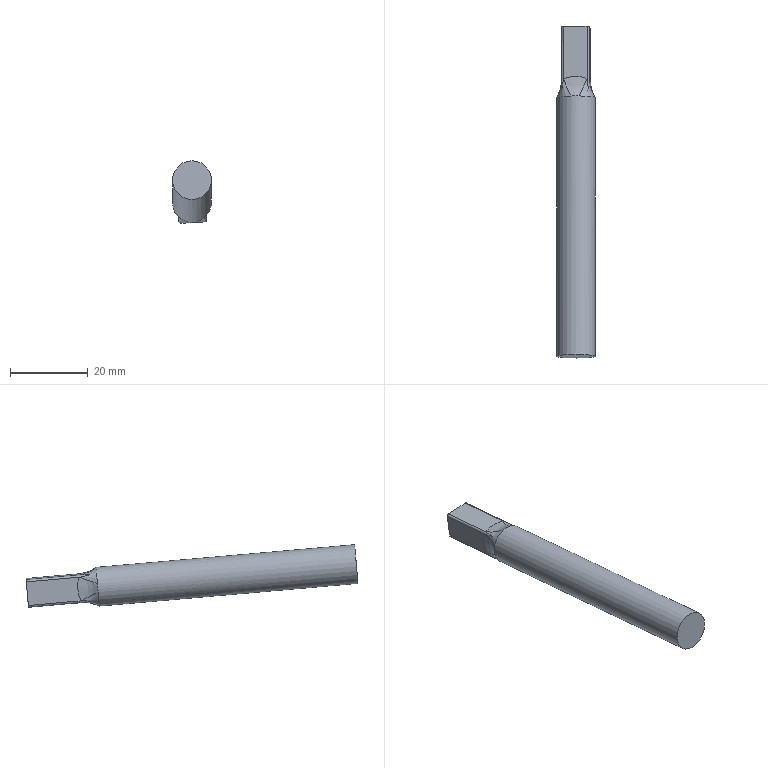Part | NX | features SPRS 10-80-7.100-7.100 2 | 1 solid | 19 faces | box 10 x 85.436 x 16.095 mm | volume 6207 mm3 | spline 8 | plane 6 | cylinder 5 | commonest cylinder face diameters 1 x4 10 x1
STEP:
#1=CARTESIAN_POINT('',(-225.118,-53.512,-35.743));
#2=VERTEX_POINT('',#1);
#3=CARTESIAN_POINT('',(-225.118,-67.066,-34.557));
#4=VERTEX_POINT('',#3);
#5=CARTESIAN_POINT('',(-225.118,-71.629,-34.158));
#6=DIRECTION('',(0.,0.9962,-0.08716));
#7=VECTOR('',#6,1000.);
#8=LINE('',#5,#7);
#9=EDGE_CURVE('',#2,#4,#8,.F.);
#10=ORIENTED_EDGE('',*,*,#9,.T.);
#11=CARTESIAN_POINT('',(-231.208,-67.096,-34.904));
#12=VERTEX_POINT('',#11);
#13=CARTESIAN_POINT('',(-225.118,-67.066,-34.557));
#14=CARTESIAN_POINT('',(-227.051,-66.254,-34.739));
#15=CARTESIAN_POINT('',(-229.277,-66.265,-34.866));
#16=CARTESIAN_POINT('',(-231.208,-67.096,-34.904));
#17=B_SPLINE_CURVE_WITH_KNOTS('',3,(#13,#14,#15,#16),.UNSPECIFIED.,.F.,.F.,(4,4),(0.,0.006313),.UNSPECIFIED.);
#18=EDGE_CURVE('',#4,#12,#17,.T.);
#19=ORIENTED_EDGE('',*,*,#18,.T.);
#20=CARTESIAN_POINT('',(-231.208,-53.543,-36.09));
#21=VERTEX_POINT('',#20);
#22=CARTESIAN_POINT('',(-231.208,-71.66,-34.505));
#23=DIRECTION('',(0.,0.9962,-0.08716));
#24=VECTOR('',#23,1000.);
#25=LINE('',#22,#24);
#26=EDGE_CURVE('',#12,#21,#25,.T.);
#27=ORIENTED_EDGE('',*,*,#26,.T.);
#28=CARTESIAN_POINT('',(-231.708,-53.545,-36.119));
#29=DIRECTION('',(0.9984,0.004985,0.05697));
#30=VECTOR('',#29,1000.);
#31=LINE('',#28,#30);
#32=EDGE_CURVE('',#21,#2,#31,.T.);
#33=ORIENTED_EDGE('',*,*,#32,.T.);
#34=EDGE_LOOP('',(#10,#19,#27,#33));
#35=FACE_BOUND('',#34,.T.);
#36=CARTESIAN_POINT('',(-231.708,-71.662,-34.534));
#37=DIRECTION('',(-0.05719,0.08701,0.9946));
#38=DIRECTION('',(0.,-0.9962,0.08716));
#39=AXIS2_PLACEMENT_3D('',#36,#37,#38);
#40=PLANE('',#39);
#41=ADVANCED_FACE('',(#35),#40,.F.);
#42=CARTESIAN_POINT('',(-224.997,-52.935,-29.15));
#43=VERTEX_POINT('',#42);
#44=CARTESIAN_POINT('',(-224.997,-66.489,-27.964));
#45=VERTEX_POINT('',#44);
#46=CARTESIAN_POINT('',(-224.997,-71.053,-27.565));
#47=DIRECTION('',(0.,0.9962,-0.08716));
#48=VECTOR('',#47,1000.);
#49=LINE('',#46,#48);
#50=EDGE_CURVE('',#43,#45,#49,.F.);
#51=ORIENTED_EDGE('',*,*,#50,.T.);
#52=CARTESIAN_POINT('',(-224.648,-67.02,-34.031));
#53=VERTEX_POINT('',#52);
#54=CARTESIAN_POINT('',(-224.997,-66.489,-27.964));
#55=CARTESIAN_POINT('',(-224.886,-65.836,-29.962));
#56=CARTESIAN_POINT('',(-224.758,-66.03,-32.179));
#57=CARTESIAN_POINT('',(-224.648,-67.02,-34.031));
#58=B_SPLINE_CURVE_WITH_KNOTS('',3,(#54,#55,#56,#57),.UNSPECIFIED.,.F.,.F.,(4,4),(0.,0.006313),.UNSPECIFIED.);
#59=EDGE_CURVE('',#45,#53,#58,.T.);
#60=ORIENTED_EDGE('',*,*,#59,.T.);
#61=CARTESIAN_POINT('',(-224.648,-53.466,-35.217));
#62=VERTEX_POINT('',#61);
#63=CARTESIAN_POINT('',(-224.648,-53.466,-35.217));
#64=DIRECTION('',(0.,0.9962,-0.08716));
#65=VECTOR('',#64,1000.);
#66=LINE('',#63,#65);
#67=EDGE_CURVE('',#53,#62,#66,.T.);
#68=ORIENTED_EDGE('',*,*,#67,.T.);
#69=CARTESIAN_POINT('',(-225.025,-52.892,-28.653));
#70=DIRECTION('',(0.05719,-0.08701,-0.9946));
#71=VECTOR('',#70,1000.);
#72=LINE('',#69,#71);
#73=EDGE_CURVE('',#43,#62,#72,.T.);
#74=ORIENTED_EDGE('',*,*,#73,.F.);
#75=EDGE_LOOP('',(#51,#60,#68,#74));
#76=FACE_BOUND('',#75,.T.);
#77=CARTESIAN_POINT('',(-225.025,-71.009,-27.068));
#78=DIRECTION('',(0.9984,0.004985,0.05697));
#79=DIRECTION('',(0.05698,0.,-0.9984));
#80=AXIS2_PLACEMENT_3D('',#77,#78,#79);
#81=PLANE('',#80);
#82=ADVANCED_FACE('',(#76),#81,.T.);
#83=CARTESIAN_POINT('',(-231.614,-52.925,-29.029));
#84=VERTEX_POINT('',#83);
#85=CARTESIAN_POINT('',(-231.614,-66.478,-27.843));
#86=VERTEX_POINT('',#85);
#87=CARTESIAN_POINT('',(-231.614,-71.042,-27.444));
#88=DIRECTION('',(0.,0.9962,-0.08716));
#89=VECTOR('',#88,1000.);
#90=LINE('',#87,#89);
#91=EDGE_CURVE('',#84,#86,#90,.F.);
#92=ORIENTED_EDGE('',*,*,#91,.T.);
#93=CARTESIAN_POINT('',(-225.524,-66.448,-27.495));
#94=VERTEX_POINT('',#93);
#95=CARTESIAN_POINT('',(-231.614,-66.478,-27.843));
#96=CARTESIAN_POINT('',(-229.682,-65.647,-27.805));
#97=CARTESIAN_POINT('',(-227.456,-65.636,-27.678));
#98=CARTESIAN_POINT('',(-225.524,-66.448,-27.495));
#99=B_SPLINE_CURVE_WITH_KNOTS('',3,(#95,#96,#97,#98),.UNSPECIFIED.,.F.,.F.,(4,4),(0.,0.006313),.UNSPECIFIED.);
#100=EDGE_CURVE('',#86,#94,#99,.T.);
#101=ORIENTED_EDGE('',*,*,#100,.T.);
#102=CARTESIAN_POINT('',(-225.524,-52.894,-28.681));
#103=VERTEX_POINT('',#102);
#104=CARTESIAN_POINT('',(-225.524,-52.894,-28.681));
#105=DIRECTION('',(0.,0.9962,-0.08716));
#106=VECTOR('',#105,1000.);
#107=LINE('',#104,#106);
#108=EDGE_CURVE('',#94,#103,#107,.T.);
#109=ORIENTED_EDGE('',*,*,#108,.T.);
#110=CARTESIAN_POINT('',(-225.025,-52.892,-28.653));
#111=DIRECTION('',(-0.9984,-0.004985,-0.05697));
#112=VECTOR('',#111,1000.);
#113=LINE('',#110,#112);
#114=EDGE_CURVE('',#103,#84,#113,.T.);
#115=ORIENTED_EDGE('',*,*,#114,.T.);
#116=EDGE_LOOP('',(#92,#101,#109,#115));
#117=FACE_BOUND('',#116,.T.);
#118=CARTESIAN_POINT('',(-225.025,-71.009,-27.068));
#119=DIRECTION('',(0.05719,-0.08701,-0.9946));
#120=DIRECTION('',(0.,0.9962,-0.08716));
#121=AXIS2_PLACEMENT_3D('',#118,#119,#120);
#122=PLANE('',#121);
#123=ADVANCED_FACE('',(#117),#122,.F.);
#124=CARTESIAN_POINT('',(-231.736,-53.502,-35.621));
#125=VERTEX_POINT('',#124);
#126=CARTESIAN_POINT('',(-231.736,-67.055,-34.436));
#127=VERTEX_POINT('',#126);
#128=CARTESIAN_POINT('',(-231.736,-71.619,-34.036));
#129=DIRECTION('',(0.,0.9962,-0.08716));
#130=VECTOR('',#129,1000.);
#131=LINE('',#128,#130);
#132=EDGE_CURVE('',#125,#127,#131,.F.);
#133=ORIENTED_EDGE('',*,*,#132,.T.);
#134=CARTESIAN_POINT('',(-232.085,-66.524,-28.369));
#135=VERTEX_POINT('',#134);
#136=CARTESIAN_POINT('',(-231.736,-67.055,-34.436));
#137=CARTESIAN_POINT('',(-231.847,-66.065,-32.582));
#138=CARTESIAN_POINT('',(-231.974,-65.872,-30.365));
#139=CARTESIAN_POINT('',(-232.085,-66.524,-28.369));
#140=B_SPLINE_CURVE_WITH_KNOTS('',3,(#136,#137,#138,#139),.UNSPECIFIED.,.F.,.F.,(4,4),(0.,0.006313),.UNSPECIFIED.);
#141=EDGE_CURVE('',#127,#135,#140,.T.);
#142=ORIENTED_EDGE('',*,*,#141,.T.);
#143=CARTESIAN_POINT('',(-232.085,-52.971,-29.555));
#144=VERTEX_POINT('',#143);
#145=CARTESIAN_POINT('',(-232.085,-71.088,-27.97));
#146=DIRECTION('',(0.,0.9962,-0.08716));
#147=VECTOR('',#146,1000.);
#148=LINE('',#145,#147);
#149=EDGE_CURVE('',#135,#144,#148,.T.);
#150=ORIENTED_EDGE('',*,*,#149,.T.);
#151=CARTESIAN_POINT('',(-232.114,-52.927,-29.057));
#152=DIRECTION('',(0.05719,-0.08701,-0.9946));
#153=VECTOR('',#152,1000.);
#154=LINE('',#151,#153);
#155=EDGE_CURVE('',#144,#125,#154,.T.);
#156=ORIENTED_EDGE('',*,*,#155,.T.);
#157=EDGE_LOOP('',(#133,#142,#150,#156));
#158=FACE_BOUND('',#157,.T.);
#159=CARTESIAN_POINT('',(-232.114,-71.044,-27.472));
#160=DIRECTION('',(0.9984,0.004985,0.05697));
#161=DIRECTION('',(0.05698,0.,-0.9984));
#162=AXIS2_PLACEMENT_3D('',#159,#160,#161);
#163=PLANE('',#162);
#164=ADVANCED_FACE('',(#158),#163,.F.);
#165=ORIENTED_EDGE('',*,*,#73,.T.);
#166=CARTESIAN_POINT('',(-225.147,-53.469,-35.245));
#167=DIRECTION('',(0.,0.9962,-0.08716));
#168=DIRECTION('',(0.,0.08716,0.9962));
#169=AXIS2_PLACEMENT_3D('',#166,#167,#168);
#170=CIRCLE('',#169,0.5);
#171=EDGE_CURVE('',#62,#2,#170,.T.);
#172=ORIENTED_EDGE('',*,*,#171,.T.);
#173=ORIENTED_EDGE('',*,*,#32,.F.);
#174=CARTESIAN_POINT('',(-231.237,-53.499,-35.593));
#175=DIRECTION('',(0.,0.9962,-0.08716));
#176=DIRECTION('',(0.,0.08716,0.9962));
#177=AXIS2_PLACEMENT_3D('',#174,#175,#176);
#178=CIRCLE('',#177,0.5);
#179=EDGE_CURVE('',#21,#125,#178,.T.);
#180=ORIENTED_EDGE('',*,*,#179,.T.);
#181=ORIENTED_EDGE('',*,*,#155,.F.);
#182=CARTESIAN_POINT('',(-231.586,-52.968,-29.526));
#183=DIRECTION('',(0.,0.9962,-0.08716));
#184=DIRECTION('',(0.,0.08716,0.9962));
#185=AXIS2_PLACEMENT_3D('',#182,#183,#184);
#186=CIRCLE('',#185,0.5);
#187=EDGE_CURVE('',#144,#84,#186,.T.);
#188=ORIENTED_EDGE('',*,*,#187,.T.);
#189=ORIENTED_EDGE('',*,*,#114,.F.);
#190=CARTESIAN_POINT('',(-225.496,-52.938,-29.179));
#191=DIRECTION('',(0.,0.9962,-0.08716));
#192=DIRECTION('',(0.,0.08716,0.9962));
#193=AXIS2_PLACEMENT_3D('',#190,#191,#192);
#194=CIRCLE('',#193,0.5);
#195=EDGE_CURVE('',#103,#43,#194,.T.);
#196=ORIENTED_EDGE('',*,*,#195,.T.);
#197=EDGE_LOOP('',(#165,#172,#173,#180,#181,#188,#189,#196));
#198=FACE_BOUND('',#197,.T.);
#199=CARTESIAN_POINT('',(-231.708,-53.545,-36.119));
#200=DIRECTION('',(0.,0.9962,-0.08716));
#201=DIRECTION('',(0.,0.08716,0.9962));
#202=AXIS2_PLACEMENT_3D('',#199,#200,#201);
#203=PLANE('',#202);
#204=ADVANCED_FACE('',(#198),#203,.T.);
#205=CARTESIAN_POINT('',(-228.366,-138.331,-29.958));
#206=VERTEX_POINT('',#205);
#207=CARTESIAN_POINT('',(-228.366,-137.895,-24.977));
#208=DIRECTION('',(0.,-0.9962,0.08716));
#209=DIRECTION('',(0.,-0.08716,-0.9962));
#210=AXIS2_PLACEMENT_3D('',#207,#208,#209);
#211=CIRCLE('',#210,5.);
#212=EDGE_CURVE('',#206,#206,#211,.F.);
#213=ORIENTED_EDGE('',*,*,#212,.F.);
#214=EDGE_LOOP('',(#213));
#215=FACE_BOUND('',#214,.T.);
#216=CARTESIAN_POINT('',(-228.366,-137.895,-24.977));
#217=DIRECTION('',(0.,-0.9962,0.08716));
#218=DIRECTION('',(0.,-0.08716,-0.9962));
#219=AXIS2_PLACEMENT_3D('',#216,#217,#218);
#220=PLANE('',#219);
#221=ADVANCED_FACE('',(#215),#220,.T.);
#222=ORIENTED_EDGE('',*,*,#212,.T.);
#223=EDGE_LOOP('',(#222));
#224=FACE_BOUND('',#223,.T.);
#225=CARTESIAN_POINT('',(-226.991,-71.755,-35.59));
#226=VERTEX_POINT('',#225);
#227=CARTESIAN_POINT('',(-223.434,-71.407,-31.615));
#228=VERTEX_POINT('',#227);
#229=CARTESIAN_POINT('',(-228.366,-71.336,-30.801));
#230=DIRECTION('',(0.,-0.9962,0.08716));
#231=DIRECTION('',(0.,-0.08716,-0.9962));
#232=AXIS2_PLACEMENT_3D('',#229,#230,#231);
#233=CIRCLE('',#232,5.);
#234=EDGE_CURVE('',#226,#228,#233,.T.);
#235=ORIENTED_EDGE('',*,*,#234,.T.);
#236=CARTESIAN_POINT('',(-223.559,-71.216,-29.431));
#237=VERTEX_POINT('',#236);
#238=CARTESIAN_POINT('',(-228.366,-71.336,-30.801));
#239=DIRECTION('',(0.,-0.9962,0.08716));
#240=DIRECTION('',(0.,-0.08716,-0.9962));
#241=AXIS2_PLACEMENT_3D('',#238,#239,#240);
#242=CIRCLE('',#241,5.);
#243=EDGE_CURVE('',#228,#237,#242,.T.);
#244=ORIENTED_EDGE('',*,*,#243,.T.);
#245=CARTESIAN_POINT('',(-227.549,-70.906,-25.887));
#246=VERTEX_POINT('',#245);
#247=CARTESIAN_POINT('',(-228.366,-71.336,-30.801));
#248=DIRECTION('',(0.,-0.9962,0.08716));
#249=DIRECTION('',(0.,-0.08716,-0.9962));
#250=AXIS2_PLACEMENT_3D('',#247,#248,#249);
#251=CIRCLE('',#250,5.);
#252=EDGE_CURVE('',#237,#246,#251,.T.);
#253=ORIENTED_EDGE('',*,*,#252,.T.);
#254=CARTESIAN_POINT('',(-229.742,-70.917,-26.012));
#255=VERTEX_POINT('',#254);
#256=CARTESIAN_POINT('',(-228.366,-71.336,-30.801));
#257=DIRECTION('',(0.,-0.9962,0.08716));
#258=DIRECTION('',(0.,-0.08716,-0.9962));
#259=AXIS2_PLACEMENT_3D('',#256,#257,#258);
#260=CIRCLE('',#259,5.);
#261=EDGE_CURVE('',#246,#255,#260,.T.);
#262=ORIENTED_EDGE('',*,*,#261,.T.);
#263=CARTESIAN_POINT('',(-233.299,-71.264,-29.987));
#264=VERTEX_POINT('',#263);
#265=CARTESIAN_POINT('',(-228.366,-71.336,-30.801));
#266=DIRECTION('',(0.,-0.9962,0.08716));
#267=DIRECTION('',(0.,-0.08716,-0.9962));
#268=AXIS2_PLACEMENT_3D('',#265,#266,#267);
#269=CIRCLE('',#268,5.);
#270=EDGE_CURVE('',#255,#264,#269,.T.);
#271=ORIENTED_EDGE('',*,*,#270,.T.);
#272=CARTESIAN_POINT('',(-233.174,-71.455,-32.171));
#273=VERTEX_POINT('',#272);
#274=CARTESIAN_POINT('',(-228.366,-71.336,-30.801));
#275=DIRECTION('',(0.,-0.9962,0.08716));
#276=DIRECTION('',(0.,-0.08716,-0.9962));
#277=AXIS2_PLACEMENT_3D('',#274,#275,#276);
#278=CIRCLE('',#277,5.);
#279=EDGE_CURVE('',#264,#273,#278,.T.);
#280=ORIENTED_EDGE('',*,*,#279,.T.);
#281=CARTESIAN_POINT('',(-229.184,-71.766,-35.715));
#282=VERTEX_POINT('',#281);
#283=CARTESIAN_POINT('',(-228.366,-71.336,-30.801));
#284=DIRECTION('',(0.,-0.9962,0.08716));
#285=DIRECTION('',(0.,-0.08716,-0.9962));
#286=AXIS2_PLACEMENT_3D('',#283,#284,#285);
#287=CIRCLE('',#286,5.);
#288=EDGE_CURVE('',#273,#282,#287,.T.);
#289=ORIENTED_EDGE('',*,*,#288,.T.);
#290=CARTESIAN_POINT('',(-228.366,-71.336,-30.801));
#291=DIRECTION('',(0.,-0.9962,0.08716));
#292=DIRECTION('',(0.,-0.08716,-0.9962));
#293=AXIS2_PLACEMENT_3D('',#290,#291,#292);
#294=CIRCLE('',#293,5.);
#295=EDGE_CURVE('',#282,#226,#294,.T.);
#296=ORIENTED_EDGE('',*,*,#295,.T.);
#297=EDGE_LOOP('',(#235,#244,#253,#262,#271,#280,#289,#296));
#298=FACE_BOUND('',#297,.T.);
#299=CARTESIAN_POINT('',(-228.366,-71.336,-30.801));
#300=DIRECTION('',(0.,-0.9962,0.08716));
#301=DIRECTION('',(0.,-0.08716,-0.9962));
#302=AXIS2_PLACEMENT_3D('',#299,#300,#301);
#303=CYLINDRICAL_SURFACE('',#302,5.);
#304=ADVANCED_FACE('',(#224,#298),#303,.T.);
#305=ORIENTED_EDGE('',*,*,#67,.F.);
#306=CARTESIAN_POINT('',(-224.648,-67.02,-34.031));
#307=CARTESIAN_POINT('',(-224.646,-67.246,-34.036));
#308=CARTESIAN_POINT('',(-224.647,-67.698,-34.047));
#309=CARTESIAN_POINT('',(-224.658,-68.262,-34.061));
#310=CARTESIAN_POINT('',(-224.673,-68.715,-34.074));
#311=CARTESIAN_POINT('',(-224.688,-69.05,-34.084));
#312=CARTESIAN_POINT('',(-224.711,-69.342,-34.102));
#313=CARTESIAN_POINT('',(-224.724,-69.546,-34.11));
#314=CARTESIAN_POINT('',(-224.783,-69.775,-34.167));
#315=CARTESIAN_POINT('',(-224.83,-69.528,-34.229));
#316=CARTESIAN_POINT('',(-224.86,-69.34,-34.268));
#317=CARTESIAN_POINT('',(-224.896,-69.051,-34.317));
#318=CARTESIAN_POINT('',(-224.934,-68.726,-34.365));
#319=CARTESIAN_POINT('',(-224.984,-68.283,-34.425));
#320=CARTESIAN_POINT('',(-225.044,-67.731,-34.491));
#321=CARTESIAN_POINT('',(-225.094,-67.287,-34.536));
#322=CARTESIAN_POINT('',(-225.118,-67.066,-34.557));
#323=B_SPLINE_CURVE_WITH_KNOTS('',3,(#306,#307,#308,#309,#310,#311,#312,#313,#314,#315,#316,#317,#318,#319,#320,#321,#322),.UNSPECIFIED.,.F.,.F.,(4,1,1,1,1,1,1,1,1,1,1,1,1,1,4),(0.,0.0006782,0.001356,0.001695,0.002035,0.002374,0.002543,0.002713,0.002882,0.003052,0.003391,0.00373,0.004069,0.004747,0.005425),.UNSPECIFIED.);
#324=EDGE_CURVE('',#53,#4,#323,.T.);
#325=ORIENTED_EDGE('',*,*,#324,.T.);
#326=ORIENTED_EDGE('',*,*,#9,.F.);
#327=ORIENTED_EDGE('',*,*,#171,.F.);
#328=EDGE_LOOP('',(#305,#325,#326,#327));
#329=FACE_BOUND('',#328,.T.);
#330=CARTESIAN_POINT('',(-225.147,-71.586,-33.66));
#331=DIRECTION('',(0.,-0.9962,0.08716));
#332=DIRECTION('',(0.,-0.08716,-0.9962));
#333=AXIS2_PLACEMENT_3D('',#330,#331,#332);
#334=CYLINDRICAL_SURFACE('',#333,0.5);
#335=ADVANCED_FACE('',(#329),#334,.T.);
#336=ORIENTED_EDGE('',*,*,#108,.F.);
#337=CARTESIAN_POINT('',(-225.524,-66.448,-27.495));
#338=CARTESIAN_POINT('',(-225.499,-66.672,-27.474));
#339=CARTESIAN_POINT('',(-225.449,-67.12,-27.436));
#340=CARTESIAN_POINT('',(-225.387,-67.679,-27.398));
#341=CARTESIAN_POINT('',(-225.334,-68.129,-27.374));
#342=CARTESIAN_POINT('',(-225.295,-68.462,-27.359));
#343=CARTESIAN_POINT('',(-225.252,-68.752,-27.357));
#344=CARTESIAN_POINT('',(-225.226,-68.954,-27.353));
#345=CARTESIAN_POINT('',(-225.149,-69.183,-27.392));
#346=CARTESIAN_POINT('',(-225.109,-68.935,-27.461));
#347=CARTESIAN_POINT('',(-225.086,-68.748,-27.507));
#348=CARTESIAN_POINT('',(-225.062,-68.461,-27.569));
#349=CARTESIAN_POINT('',(-225.043,-68.137,-27.635));
#350=CARTESIAN_POINT('',(-225.022,-67.697,-27.723));
#351=CARTESIAN_POINT('',(-225.005,-67.148,-27.832));
#352=CARTESIAN_POINT('',(-224.998,-66.709,-27.92));
#353=CARTESIAN_POINT('',(-224.997,-66.489,-27.964));
#354=B_SPLINE_CURVE_WITH_KNOTS('',3,(#337,#338,#339,#340,#341,#342,#343,#344,#345,#346,#347,#348,#349,#350,#351,#352,#353),.UNSPECIFIED.,.F.,.F.,(4,1,1,1,1,1,1,1,1,1,1,1,1,1,4),(0.,0.0006782,0.001356,0.001695,0.002035,0.002374,0.002543,0.002713,0.002882,0.003052,0.003391,0.00373,0.004069,0.004747,0.005425),.UNSPECIFIED.);
#355=EDGE_CURVE('',#94,#45,#354,.T.);
#356=ORIENTED_EDGE('',*,*,#355,.T.);
#357=ORIENTED_EDGE('',*,*,#50,.F.);
#358=ORIENTED_EDGE('',*,*,#195,.F.);
#359=EDGE_LOOP('',(#336,#356,#357,#358));
#360=FACE_BOUND('',#359,.T.);
#361=CARTESIAN_POINT('',(-225.496,-71.055,-27.593));
#362=DIRECTION('',(0.,-0.9962,0.08716));
#363=DIRECTION('',(0.,-0.08716,-0.9962));
#364=AXIS2_PLACEMENT_3D('',#361,#362,#363);
#365=CYLINDRICAL_SURFACE('',#364,0.5);
#366=ADVANCED_FACE('',(#360),#365,.T.);
#367=ORIENTED_EDGE('',*,*,#26,.F.);
#368=CARTESIAN_POINT('',(-231.208,-67.096,-34.904));
#369=CARTESIAN_POINT('',(-231.233,-67.32,-34.886));
#370=CARTESIAN_POINT('',(-231.284,-67.768,-34.846));
#371=CARTESIAN_POINT('',(-231.346,-68.326,-34.787));
#372=CARTESIAN_POINT('',(-231.399,-68.773,-34.732));
#373=CARTESIAN_POINT('',(-231.438,-69.103,-34.689));
#374=CARTESIAN_POINT('',(-231.481,-69.389,-34.64));
#375=CARTESIAN_POINT('',(-231.507,-69.589,-34.61));
#376=CARTESIAN_POINT('',(-231.584,-69.807,-34.531));
#377=CARTESIAN_POINT('',(-231.624,-69.552,-34.507));
#378=CARTESIAN_POINT('',(-231.647,-69.36,-34.494));
#379=CARTESIAN_POINT('',(-231.671,-69.066,-34.483));
#380=CARTESIAN_POINT('',(-231.69,-68.735,-34.474));
#381=CARTESIAN_POINT('',(-231.711,-68.286,-34.463));
#382=CARTESIAN_POINT('',(-231.728,-67.727,-34.451));
#383=CARTESIAN_POINT('',(-231.735,-67.279,-34.441));
#384=CARTESIAN_POINT('',(-231.736,-67.055,-34.436));
#385=B_SPLINE_CURVE_WITH_KNOTS('',3,(#368,#369,#370,#371,#372,#373,#374,#375,#376,#377,#378,#379,#380,#381,#382,#383,#384),.UNSPECIFIED.,.F.,.F.,(4,1,1,1,1,1,1,1,1,1,1,1,1,1,4),(0.,0.0006782,0.001356,0.001695,0.002035,0.002374,0.002543,0.002713,0.002882,0.003052,0.003391,0.00373,0.004069,0.004747,0.005425),.UNSPECIFIED.);
#386=EDGE_CURVE('',#12,#127,#385,.T.);
#387=ORIENTED_EDGE('',*,*,#386,.T.);
#388=ORIENTED_EDGE('',*,*,#132,.F.);
#389=ORIENTED_EDGE('',*,*,#179,.F.);
#390=EDGE_LOOP('',(#367,#387,#388,#389));
#391=FACE_BOUND('',#390,.T.);
#392=CARTESIAN_POINT('',(-231.237,-71.616,-34.008));
#393=DIRECTION('',(0.,0.9962,-0.08716));
#394=DIRECTION('',(0.,0.08716,0.9962));
#395=AXIS2_PLACEMENT_3D('',#392,#393,#394);
#396=CYLINDRICAL_SURFACE('',#395,0.5);
#397=ADVANCED_FACE('',(#391),#396,.T.);
#398=ORIENTED_EDGE('',*,*,#149,.F.);
#399=CARTESIAN_POINT('',(-232.085,-66.524,-28.369));
#400=CARTESIAN_POINT('',(-232.086,-66.746,-28.324));
#401=CARTESIAN_POINT('',(-232.086,-67.189,-28.235));
#402=CARTESIAN_POINT('',(-232.075,-67.743,-28.124));
#403=CARTESIAN_POINT('',(-232.059,-68.186,-28.032));
#404=CARTESIAN_POINT('',(-232.045,-68.515,-27.964));
#405=CARTESIAN_POINT('',(-232.022,-68.799,-27.896));
#406=CARTESIAN_POINT('',(-232.009,-68.998,-27.853));
#407=CARTESIAN_POINT('',(-231.949,-69.215,-27.756));
#408=CARTESIAN_POINT('',(-231.903,-68.96,-27.738));
#409=CARTESIAN_POINT('',(-231.873,-68.768,-27.732));
#410=CARTESIAN_POINT('',(-231.836,-68.475,-27.734));
#411=CARTESIAN_POINT('',(-231.799,-68.146,-27.743));
#412=CARTESIAN_POINT('',(-231.749,-67.7,-27.762));
#413=CARTESIAN_POINT('',(-231.689,-67.145,-27.793));
#414=CARTESIAN_POINT('',(-231.639,-66.7,-27.825));
#415=CARTESIAN_POINT('',(-231.614,-66.478,-27.843));
#416=B_SPLINE_CURVE_WITH_KNOTS('',3,(#399,#400,#401,#402,#403,#404,#405,#406,#407,#408,#409,#410,#411,#412,#413,#414,#415),.UNSPECIFIED.,.F.,.F.,(4,1,1,1,1,1,1,1,1,1,1,1,1,1,4),(0.,0.0006782,0.001356,0.001695,0.002035,0.002374,0.002543,0.002713,0.002882,0.003052,0.003391,0.00373,0.004069,0.004747,0.005425),.UNSPECIFIED.);
#417=EDGE_CURVE('',#135,#86,#416,.T.);
#418=ORIENTED_EDGE('',*,*,#417,.T.);
#419=ORIENTED_EDGE('',*,*,#91,.F.);
#420=ORIENTED_EDGE('',*,*,#187,.F.);
#421=EDGE_LOOP('',(#398,#418,#419,#420));
#422=FACE_BOUND('',#421,.T.);
#423=CARTESIAN_POINT('',(-231.586,-71.085,-27.941));
#424=DIRECTION('',(0.,0.9962,-0.08716));
#425=DIRECTION('',(0.,0.08716,0.9962));
#426=AXIS2_PLACEMENT_3D('',#423,#424,#425);
#427=CYLINDRICAL_SURFACE('',#426,0.5);
#428=ADVANCED_FACE('',(#422),#427,.T.);
#429=CARTESIAN_POINT('',(-232.186,-65.608,-17.897));
#430=DIRECTION('',(-0.9185,-0.3951,-0.01825));
#431=DIRECTION('',(0.3952,-0.9186,0.));
#432=AXIS2_PLACEMENT_3D('',#429,#430,#431);
#433=CIRCLE('',#432,10.);
#434=EDGE_CURVE('',#86,#255,#433,.T.);
#435=ORIENTED_EDGE('',*,*,#434,.F.);
#436=ORIENTED_EDGE('',*,*,#417,.F.);
#437=CARTESIAN_POINT('',(-242.069,-66.574,-28.939));
#438=DIRECTION('',(0.05261,0.3105,-0.9491));
#439=DIRECTION('',(0.,0.9504,0.3109));
#440=AXIS2_PLACEMENT_3D('',#437,#438,#439);
#441=CIRCLE('',#440,10.);
#442=EDGE_CURVE('',#264,#135,#441,.F.);
#443=ORIENTED_EDGE('',*,*,#442,.F.);
#444=ORIENTED_EDGE('',*,*,#270,.F.);
#445=EDGE_LOOP('',(#435,#436,#443,#444));
#446=FACE_BOUND('',#445,.T.);
#447=CARTESIAN_POINT('',(-232.085,-66.524,-28.369));
#448=CARTESIAN_POINT('',(-232.025,-69.059,-29.195));
#449=CARTESIAN_POINT('',(-233.299,-71.264,-29.987));
#450=CARTESIAN_POINT('',(-232.089,-67.083,-28.257));
#451=CARTESIAN_POINT('',(-232.168,-69.257,-28.984));
#452=CARTESIAN_POINT('',(-233.223,-71.224,-29.528));
#453=CARTESIAN_POINT('',(-232.072,-68.223,-28.029));
#454=CARTESIAN_POINT('',(-232.331,-69.713,-28.455));
#455=CARTESIAN_POINT('',(-232.95,-71.148,-28.655));
#456=CARTESIAN_POINT('',(-231.988,-69.378,-27.778));
#457=CARTESIAN_POINT('',(-232.089,-70.228,-27.753));
#458=CARTESIAN_POINT('',(-232.294,-71.06,-27.65));
#459=CARTESIAN_POINT('',(-231.885,-68.897,-27.726));
#460=CARTESIAN_POINT('',(-231.655,-69.969,-27.437));
#461=CARTESIAN_POINT('',(-231.585,-71.,-26.966));
#462=CARTESIAN_POINT('',(-231.772,-67.921,-27.744));
#463=CARTESIAN_POINT('',(-231.162,-69.496,-27.322));
#464=CARTESIAN_POINT('',(-230.827,-70.953,-26.423));
#465=CARTESIAN_POINT('',(-231.678,-67.046,-27.797));
#466=CARTESIAN_POINT('',(-230.78,-69.122,-27.431));
#467=CARTESIAN_POINT('',(-230.193,-70.928,-26.14));
#468=CARTESIAN_POINT('',(-231.614,-66.478,-27.843));
#469=CARTESIAN_POINT('',(-230.571,-68.917,-27.57));
#470=CARTESIAN_POINT('',(-229.742,-70.917,-26.012));
#471=(BOUNDED_SURFACE()B_SPLINE_SURFACE(3,2,((#447,#448,#449),(#450,#451,#452),(#453,#454,#455),(#456,#457,#458),(#459,#460,#461),(#462,#463,#464),(#465,#466,#467),(#468,#469,#470)),.UNSPECIFIED.,.F.,.F.,.F.)B_SPLINE_SURFACE_WITH_KNOTS((4,1,1,1,1,4),(3,3),(0.02713,0.03146,0.0358,0.03797,0.04013,0.04447),(0.,1.),.UNSPECIFIED.)GEOMETRIC_REPRESENTATION_ITEM()RATIONAL_B_SPLINE_SURFACE(((1.,0.9662,1.),(1.,0.9753,1.),(1.,0.9896,1.),(1.,0.9967,1.),(1.,0.9939,1.),(1.,0.9861,1.),(1.,0.9753,1.),(1.,0.9662,1.)))REPRESENTATION_ITEM('')SURFACE());
#472=ADVANCED_FACE('',(#446),#471,.F.);
#473=ORIENTED_EDGE('',*,*,#442,.T.);
#474=ORIENTED_EDGE('',*,*,#141,.F.);
#475=CARTESIAN_POINT('',(-241.72,-67.105,-35.005));
#476=DIRECTION('',(-0.05261,0.4706,0.8808));
#477=DIRECTION('',(0.,-0.882,0.4712));
#478=AXIS2_PLACEMENT_3D('',#475,#476,#477);
#479=CIRCLE('',#478,10.);
#480=EDGE_CURVE('',#273,#127,#479,.T.);
#481=ORIENTED_EDGE('',*,*,#480,.F.);
#482=ORIENTED_EDGE('',*,*,#279,.F.);
#483=EDGE_LOOP('',(#473,#474,#481,#482));
#484=FACE_BOUND('',#483,.T.);
#485=CARTESIAN_POINT('',(-233.299,-71.264,-29.987));
#486=CARTESIAN_POINT('',(-232.025,-69.059,-29.195));
#487=CARTESIAN_POINT('',(-232.085,-66.524,-28.369));
#488=CARTESIAN_POINT('',(-233.409,-71.322,-30.649));
#489=CARTESIAN_POINT('',(-231.953,-68.808,-30.475));
#490=CARTESIAN_POINT('',(-231.975,-65.877,-30.348));
#491=CARTESIAN_POINT('',(-233.36,-71.399,-31.521));
#492=CARTESIAN_POINT('',(-231.868,-68.935,-31.956));
#493=CARTESIAN_POINT('',(-231.847,-66.067,-32.586));
#494=CARTESIAN_POINT('',(-233.174,-71.455,-32.171));
#495=CARTESIAN_POINT('',(-231.796,-69.408,-33.182));
#496=CARTESIAN_POINT('',(-231.736,-67.055,-34.436));
#497=(BOUNDED_SURFACE()B_SPLINE_SURFACE(3,2,((#485,#486,#487),(#488,#489,#490),(#491,#492,#493),(#494,#495,#496)),.UNSPECIFIED.,.F.,.F.,.F.)B_SPLINE_SURFACE_WITH_KNOTS((4,4),(3,3),(0.005986,0.0122),(0.,1.),.PIECEWISE_BEZIER_KNOTS.)GEOMETRIC_REPRESENTATION_ITEM()RATIONAL_B_SPLINE_SURFACE(((1.,0.9662,1.),(1.,0.9624,1.),(1.,0.9624,1.),(1.,0.9662,1.)))REPRESENTATION_ITEM('')SURFACE());
#498=ADVANCED_FACE('',(#484),#497,.F.);
#499=ORIENTED_EDGE('',*,*,#434,.T.);
#500=ORIENTED_EDGE('',*,*,#261,.F.);
#501=CARTESIAN_POINT('',(-226.096,-65.578,-17.55));
#502=DIRECTION('',(0.9185,-0.3859,0.08658));
#503=DIRECTION('',(0.3874,0.9219,0.));
#504=AXIS2_PLACEMENT_3D('',#501,#502,#503);
#505=CIRCLE('',#504,10.);
#506=EDGE_CURVE('',#94,#246,#505,.F.);
#507=ORIENTED_EDGE('',*,*,#506,.F.);
#508=ORIENTED_EDGE('',*,*,#100,.F.);
#509=EDGE_LOOP('',(#499,#500,#507,#508));
#510=FACE_BOUND('',#509,.T.);
#511=CARTESIAN_POINT('',(-227.549,-70.906,-25.887));
#512=CARTESIAN_POINT('',(-226.568,-68.897,-27.341));
#513=CARTESIAN_POINT('',(-225.524,-66.448,-27.495));
#514=CARTESIAN_POINT('',(-228.214,-70.896,-25.777));
#515=CARTESIAN_POINT('',(-227.822,-68.543,-27.444));
#516=CARTESIAN_POINT('',(-227.439,-65.643,-27.676));
#517=CARTESIAN_POINT('',(-229.089,-70.9,-25.826));
#518=CARTESIAN_POINT('',(-229.308,-68.548,-27.529));
#519=CARTESIAN_POINT('',(-229.686,-65.649,-27.805));
#520=CARTESIAN_POINT('',(-229.742,-70.917,-26.012));
#521=CARTESIAN_POINT('',(-230.571,-68.917,-27.57));
#522=CARTESIAN_POINT('',(-231.614,-66.478,-27.843));
#523=(BOUNDED_SURFACE()B_SPLINE_SURFACE(3,2,((#511,#512,#513),(#514,#515,#516),(#517,#518,#519),(#520,#521,#522)),.UNSPECIFIED.,.F.,.F.,.F.)B_SPLINE_SURFACE_WITH_KNOTS((4,4),(3,3),(0.005986,0.0122),(0.,1.),.PIECEWISE_BEZIER_KNOTS.)GEOMETRIC_REPRESENTATION_ITEM()RATIONAL_B_SPLINE_SURFACE(((1.,0.9662,1.),(1.,0.9624,1.),(1.,0.9624,1.),(1.,0.9662,1.)))REPRESENTATION_ITEM('')SURFACE());
#524=ADVANCED_FACE('',(#510),#523,.F.);
#525=ORIENTED_EDGE('',*,*,#480,.T.);
#526=ORIENTED_EDGE('',*,*,#386,.F.);
#527=CARTESIAN_POINT('',(-230.636,-67.966,-44.85));
#528=DIRECTION('',(0.9185,0.3951,0.01825));
#529=DIRECTION('',(-0.3952,0.9186,0.));
#530=AXIS2_PLACEMENT_3D('',#527,#528,#529);
#531=CIRCLE('',#530,10.);
#532=EDGE_CURVE('',#282,#12,#531,.F.);
#533=ORIENTED_EDGE('',*,*,#532,.F.);
#534=ORIENTED_EDGE('',*,*,#288,.F.);
#535=EDGE_LOOP('',(#525,#526,#533,#534));
#536=FACE_BOUND('',#535,.T.);
#537=CARTESIAN_POINT('',(-231.208,-67.096,-34.904));
#538=CARTESIAN_POINT('',(-230.165,-69.535,-34.631));
#539=CARTESIAN_POINT('',(-229.184,-71.766,-35.715));
#540=CARTESIAN_POINT('',(-231.272,-67.66,-34.859));
#541=CARTESIAN_POINT('',(-230.358,-69.762,-34.754));
#542=CARTESIAN_POINT('',(-229.644,-71.759,-35.639));
#543=CARTESIAN_POINT('',(-231.399,-68.811,-34.742));
#544=CARTESIAN_POINT('',(-230.845,-70.275,-34.873));
#545=CARTESIAN_POINT('',(-230.52,-71.735,-35.367));
#546=CARTESIAN_POINT('',(-231.548,-69.971,-34.556));
#547=CARTESIAN_POINT('',(-231.499,-70.826,-34.582));
#548=CARTESIAN_POINT('',(-231.529,-71.678,-34.713));
#549=CARTESIAN_POINT('',(-231.642,-69.489,-34.494));
#550=CARTESIAN_POINT('',(-231.836,-70.558,-34.17));
#551=CARTESIAN_POINT('',(-232.216,-71.616,-34.007));
#552=CARTESIAN_POINT('',(-231.709,-68.509,-34.467));
#553=CARTESIAN_POINT('',(-231.992,-70.055,-33.719));
#554=CARTESIAN_POINT('',(-232.761,-71.55,-33.252));
#555=CARTESIAN_POINT('',(-231.733,-67.628,-34.449));
#556=CARTESIAN_POINT('',(-231.916,-69.642,-33.372));
#557=CARTESIAN_POINT('',(-233.044,-71.495,-32.62));
#558=CARTESIAN_POINT('',(-231.736,-67.055,-34.436));
#559=CARTESIAN_POINT('',(-231.796,-69.408,-33.182));
#560=CARTESIAN_POINT('',(-233.174,-71.455,-32.171));
#561=(BOUNDED_SURFACE()B_SPLINE_SURFACE(3,2,((#537,#538,#539),(#540,#541,#542),(#543,#544,#545),(#546,#547,#548),(#549,#550,#551),(#552,#553,#554),(#555,#556,#557),(#558,#559,#560)),.UNSPECIFIED.,.F.,.F.,.F.)B_SPLINE_SURFACE_WITH_KNOTS((4,1,1,1,1,4),(3,3),(0.02713,0.03146,0.0358,0.03797,0.04013,0.04447),(0.,1.),.UNSPECIFIED.)GEOMETRIC_REPRESENTATION_ITEM()RATIONAL_B_SPLINE_SURFACE(((1.,0.9662,1.),(1.,0.9753,1.),(1.,0.9896,1.),(1.,0.9967,1.),(1.,0.9939,1.),(1.,0.9861,1.),(1.,0.9753,1.),(1.,0.9662,1.)))REPRESENTATION_ITEM('')SURFACE());
#562=ADVANCED_FACE('',(#536),#561,.F.);
#563=ORIENTED_EDGE('',*,*,#506,.T.);
#564=ORIENTED_EDGE('',*,*,#252,.F.);
#565=CARTESIAN_POINT('',(-215.013,-66.439,-27.395));
#566=DIRECTION('',(-0.05261,-0.3105,0.9491));
#567=DIRECTION('',(0.,-0.9504,-0.3109));
#568=AXIS2_PLACEMENT_3D('',#565,#566,#567);
#569=CIRCLE('',#568,10.);
#570=EDGE_CURVE('',#45,#237,#569,.T.);
#571=ORIENTED_EDGE('',*,*,#570,.F.);
#572=ORIENTED_EDGE('',*,*,#355,.F.);
#573=EDGE_LOOP('',(#563,#564,#571,#572));
#574=FACE_BOUND('',#573,.T.);
#575=CARTESIAN_POINT('',(-225.524,-66.448,-27.495));
#576=CARTESIAN_POINT('',(-226.568,-68.897,-27.341));
#577=CARTESIAN_POINT('',(-227.549,-70.906,-25.887));
#578=CARTESIAN_POINT('',(-225.461,-67.012,-27.443));
#579=CARTESIAN_POINT('',(-226.375,-69.099,-27.181));
#580=CARTESIAN_POINT('',(-227.089,-70.912,-25.963));
#581=CARTESIAN_POINT('',(-225.334,-68.165,-27.358));
#582=CARTESIAN_POINT('',(-225.888,-69.584,-26.974));
#583=CARTESIAN_POINT('',(-226.213,-70.936,-26.235));
#584=CARTESIAN_POINT('',(-225.185,-69.34,-27.34));
#585=CARTESIAN_POINT('',(-225.234,-70.177,-27.165));
#586=CARTESIAN_POINT('',(-225.204,-70.993,-26.888));
#587=CARTESIAN_POINT('',(-225.091,-68.876,-27.484));
#588=CARTESIAN_POINT('',(-224.897,-69.985,-27.618));
#589=CARTESIAN_POINT('',(-224.517,-71.055,-27.595));
#590=CARTESIAN_POINT('',(-225.024,-67.916,-27.681));
#591=CARTESIAN_POINT('',(-224.741,-69.568,-28.149));
#592=CARTESIAN_POINT('',(-223.972,-71.121,-28.349));
#593=CARTESIAN_POINT('',(-225.,-67.051,-27.851));
#594=CARTESIAN_POINT('',(-224.817,-69.221,-28.563));
#595=CARTESIAN_POINT('',(-223.688,-71.176,-28.981));
#596=CARTESIAN_POINT('',(-224.997,-66.489,-27.964));
#597=CARTESIAN_POINT('',(-224.937,-69.024,-28.79));
#598=CARTESIAN_POINT('',(-223.559,-71.216,-29.431));
#599=(BOUNDED_SURFACE()B_SPLINE_SURFACE(3,2,((#575,#576,#577),(#578,#579,#580),(#581,#582,#583),(#584,#585,#586),(#587,#588,#589),(#590,#591,#592),(#593,#594,#595),(#596,#597,#598)),.UNSPECIFIED.,.F.,.F.,.F.)B_SPLINE_SURFACE_WITH_KNOTS((4,1,1,1,1,4),(3,3),(0.02713,0.03146,0.0358,0.03797,0.04013,0.04447),(0.,1.),.UNSPECIFIED.)GEOMETRIC_REPRESENTATION_ITEM()RATIONAL_B_SPLINE_SURFACE(((1.,0.9662,1.),(1.,0.9753,1.),(1.,0.9896,1.),(1.,0.9967,1.),(1.,0.9939,1.),(1.,0.9861,1.),(1.,0.9753,1.),(1.,0.9662,1.)))REPRESENTATION_ITEM('')SURFACE());
#600=ADVANCED_FACE('',(#574),#599,.F.);
#601=ORIENTED_EDGE('',*,*,#532,.T.);
#602=ORIENTED_EDGE('',*,*,#18,.F.);
#603=CARTESIAN_POINT('',(-224.546,-67.936,-44.503));
#604=DIRECTION('',(-0.9185,0.3859,-0.08658));
#605=DIRECTION('',(-0.3874,-0.9219,0.));
#606=AXIS2_PLACEMENT_3D('',#603,#604,#605);
#607=CIRCLE('',#606,10.);
#608=EDGE_CURVE('',#226,#4,#607,.T.);
#609=ORIENTED_EDGE('',*,*,#608,.F.);
#610=ORIENTED_EDGE('',*,*,#295,.F.);
#611=EDGE_LOOP('',(#601,#602,#609,#610));
#612=FACE_BOUND('',#611,.T.);
#613=CARTESIAN_POINT('',(-229.184,-71.766,-35.715));
#614=CARTESIAN_POINT('',(-230.165,-69.535,-34.631));
#615=CARTESIAN_POINT('',(-231.208,-67.096,-34.904));
#616=CARTESIAN_POINT('',(-228.519,-71.775,-35.824));
#617=CARTESIAN_POINT('',(-228.911,-69.169,-34.591));
#618=CARTESIAN_POINT('',(-229.293,-66.272,-34.866));
#619=CARTESIAN_POINT('',(-227.644,-71.771,-35.775));
#620=CARTESIAN_POINT('',(-227.425,-69.159,-34.506));
#621=CARTESIAN_POINT('',(-227.047,-66.255,-34.739));
#622=CARTESIAN_POINT('',(-226.991,-71.755,-35.59));
#623=CARTESIAN_POINT('',(-226.162,-69.515,-34.403));
#624=CARTESIAN_POINT('',(-225.118,-67.066,-34.557));
#625=(BOUNDED_SURFACE()B_SPLINE_SURFACE(3,2,((#613,#614,#615),(#616,#617,#618),(#619,#620,#621),(#622,#623,#624)),.UNSPECIFIED.,.F.,.F.,.F.)B_SPLINE_SURFACE_WITH_KNOTS((4,4),(3,3),(0.005986,0.0122),(0.,1.),.PIECEWISE_BEZIER_KNOTS.)GEOMETRIC_REPRESENTATION_ITEM()RATIONAL_B_SPLINE_SURFACE(((1.,0.9662,1.),(1.,0.9624,1.),(1.,0.9624,1.),(1.,0.9662,1.)))REPRESENTATION_ITEM('')SURFACE());
#626=ADVANCED_FACE('',(#612),#625,.F.);
#627=ORIENTED_EDGE('',*,*,#570,.T.);
#628=ORIENTED_EDGE('',*,*,#243,.F.);
#629=CARTESIAN_POINT('',(-214.664,-66.97,-33.461));
#630=DIRECTION('',(0.05261,-0.4706,-0.8808));
#631=DIRECTION('',(0.,0.882,-0.4712));
#632=AXIS2_PLACEMENT_3D('',#629,#630,#631);
#633=CIRCLE('',#632,10.);
#634=EDGE_CURVE('',#53,#228,#633,.F.);
#635=ORIENTED_EDGE('',*,*,#634,.F.);
#636=ORIENTED_EDGE('',*,*,#59,.F.);
#637=EDGE_LOOP('',(#627,#628,#635,#636));
#638=FACE_BOUND('',#637,.T.);
#639=CARTESIAN_POINT('',(-223.434,-71.407,-31.615));
#640=CARTESIAN_POINT('',(-224.708,-69.373,-32.778));
#641=CARTESIAN_POINT('',(-224.648,-67.02,-34.031));
#642=CARTESIAN_POINT('',(-223.324,-71.349,-30.953));
#643=CARTESIAN_POINT('',(-224.779,-68.903,-31.56));
#644=CARTESIAN_POINT('',(-224.757,-66.039,-32.195));
#645=CARTESIAN_POINT('',(-223.373,-71.273,-30.081));
#646=CARTESIAN_POINT('',(-224.865,-68.771,-30.08));
#647=CARTESIAN_POINT('',(-224.886,-65.837,-29.957));
#648=CARTESIAN_POINT('',(-223.559,-71.216,-29.431));
#649=CARTESIAN_POINT('',(-224.937,-69.024,-28.79));
#650=CARTESIAN_POINT('',(-224.997,-66.489,-27.964));
#651=(BOUNDED_SURFACE()B_SPLINE_SURFACE(3,2,((#639,#640,#641),(#642,#643,#644),(#645,#646,#647),(#648,#649,#650)),.UNSPECIFIED.,.F.,.F.,.F.)B_SPLINE_SURFACE_WITH_KNOTS((4,4),(3,3),(0.005986,0.0122),(0.,1.),.PIECEWISE_BEZIER_KNOTS.)GEOMETRIC_REPRESENTATION_ITEM()RATIONAL_B_SPLINE_SURFACE(((1.,0.9662,1.),(1.,0.9624,1.),(1.,0.9624,1.),(1.,0.9662,1.)))REPRESENTATION_ITEM('')SURFACE());
#652=ADVANCED_FACE('',(#638),#651,.F.);
#653=ORIENTED_EDGE('',*,*,#608,.T.);
#654=ORIENTED_EDGE('',*,*,#324,.F.);
#655=ORIENTED_EDGE('',*,*,#634,.T.);
#656=ORIENTED_EDGE('',*,*,#234,.F.);
#657=EDGE_LOOP('',(#653,#654,#655,#656));
#658=FACE_BOUND('',#657,.T.);
#659=CARTESIAN_POINT('',(-224.648,-67.02,-34.031));
#660=CARTESIAN_POINT('',(-224.708,-69.373,-32.778));
#661=CARTESIAN_POINT('',(-223.434,-71.407,-31.615));
#662=CARTESIAN_POINT('',(-224.644,-67.589,-34.045));
#663=CARTESIAN_POINT('',(-224.565,-69.604,-32.951));
#664=CARTESIAN_POINT('',(-223.51,-71.447,-32.073));
#665=CARTESIAN_POINT('',(-224.66,-68.752,-34.07));
#666=CARTESIAN_POINT('',(-224.402,-70.145,-33.393));
#667=CARTESIAN_POINT('',(-223.783,-71.523,-32.946));
#668=CARTESIAN_POINT('',(-224.745,-69.933,-34.117));
#669=CARTESIAN_POINT('',(-224.644,-70.774,-33.995));
#670=CARTESIAN_POINT('',(-224.439,-71.611,-33.951));
#671=CARTESIAN_POINT('',(-224.848,-69.468,-34.252));
#672=CARTESIAN_POINT('',(-225.078,-70.574,-34.35));
#673=CARTESIAN_POINT('',(-225.148,-71.671,-34.635));
#674=CARTESIAN_POINT('',(-224.961,-68.504,-34.404));
#675=CARTESIAN_POINT('',(-225.571,-70.128,-34.546));
#676=CARTESIAN_POINT('',(-225.905,-71.719,-35.179));
#677=CARTESIAN_POINT('',(-225.055,-67.633,-34.504));
#678=CARTESIAN_POINT('',(-225.953,-69.741,-34.503));
#679=CARTESIAN_POINT('',(-226.54,-71.743,-35.461));
#680=CARTESIAN_POINT('',(-225.118,-67.066,-34.557));
#681=CARTESIAN_POINT('',(-226.162,-69.515,-34.403));
#682=CARTESIAN_POINT('',(-226.991,-71.755,-35.59));
#683=(BOUNDED_SURFACE()B_SPLINE_SURFACE(3,2,((#659,#660,#661),(#662,#663,#664),(#665,#666,#667),(#668,#669,#670),(#671,#672,#673),(#674,#675,#676),(#677,#678,#679),(#680,#681,#682)),.UNSPECIFIED.,.F.,.F.,.F.)B_SPLINE_SURFACE_WITH_KNOTS((4,1,1,1,1,4),(3,3),(0.02713,0.03146,0.0358,0.03797,0.04013,0.04447),(0.,1.),.UNSPECIFIED.)GEOMETRIC_REPRESENTATION_ITEM()RATIONAL_B_SPLINE_SURFACE(((1.,0.9662,1.),(1.,0.9753,1.),(1.,0.9896,1.),(1.,0.9967,1.),(1.,0.9939,1.),(1.,0.9861,1.),(1.,0.9753,1.),(1.,0.9662,1.)))REPRESENTATION_ITEM('')SURFACE());
#684=ADVANCED_FACE('',(#658),#683,.F.);
#685=CLOSED_SHELL('',(#41,#82,#123,#164,#204,#221,#304,#335,#366,#397,#428,#472,#498,#524,#562,#600,#626,#652,#684));
#686=MANIFOLD_SOLID_BREP('',#685);
#687=(LENGTH_UNIT()NAMED_UNIT(*)SI_UNIT(.MILLI.,.METRE.));
#688=UNCERTAINTY_MEASURE_WITH_UNIT(LENGTH_MEASURE(0.0508),#687,'','');
#689=(NAMED_UNIT(*)PLANE_ANGLE_UNIT()SI_UNIT($,.RADIAN.));
#690=(NAMED_UNIT(*)SI_UNIT($,.STERADIAN.)SOLID_ANGLE_UNIT());
#691=(GEOMETRIC_REPRESENTATION_CONTEXT(3)GLOBAL_UNCERTAINTY_ASSIGNED_CONTEXT((#688))GLOBAL_UNIT_ASSIGNED_CONTEXT((#687,#689,#690))REPRESENTATION_CONTEXT('',''));
#692=ADVANCED_BREP_SHAPE_REPRESENTATION('',(#686),#691);